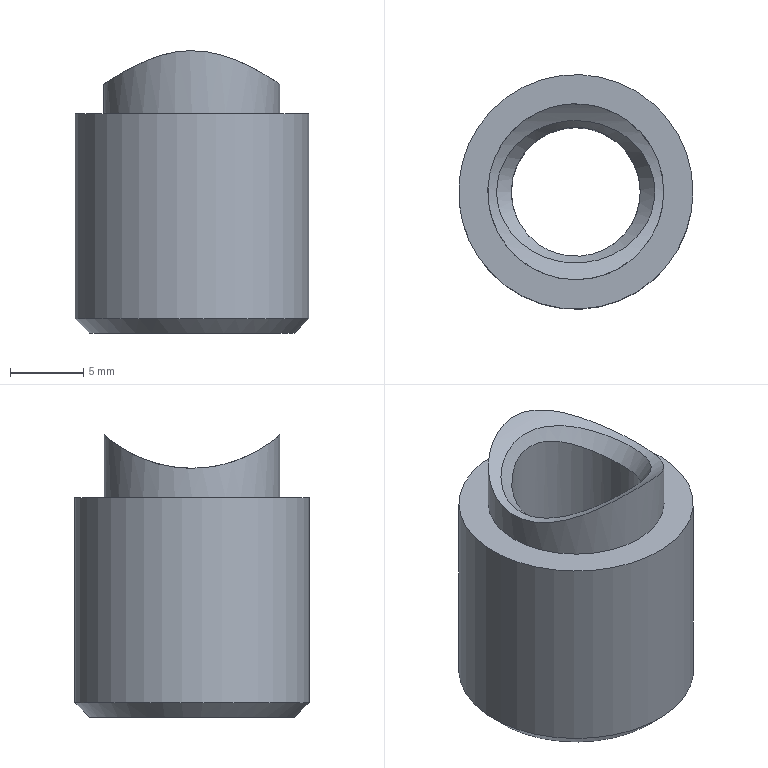Part | STEP file | JBJ-P-1012-07 | 1 solid | 9 faces | box 16 x 16 x 19.292 mm | volume 2215 mm3 | cylinder 4 | plane 2 | cone 2 | spline 1 | commonest cylinder face diameters 8.8 x1 12 x1 16 x1 18 x1